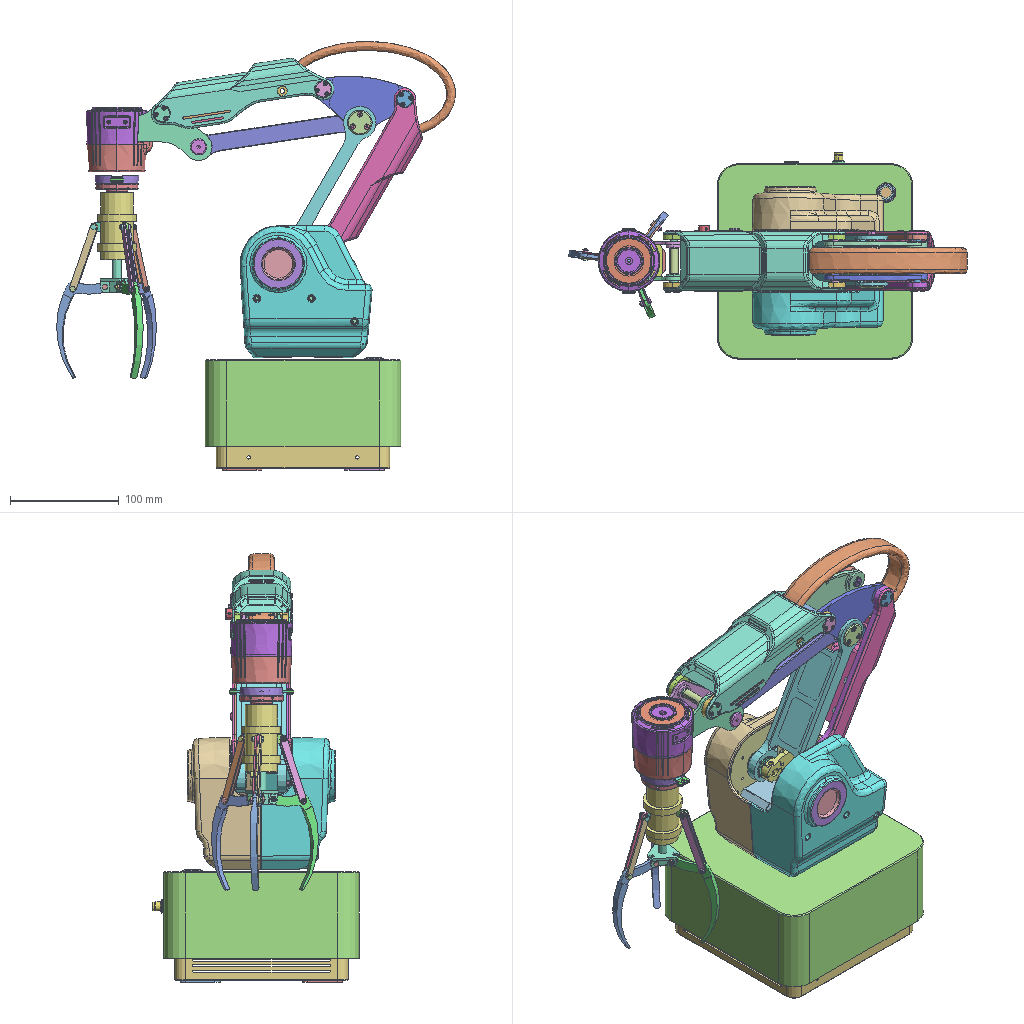Assembly | NX | 116 different items | 163 placed | box 367 x 190 x 394 mm
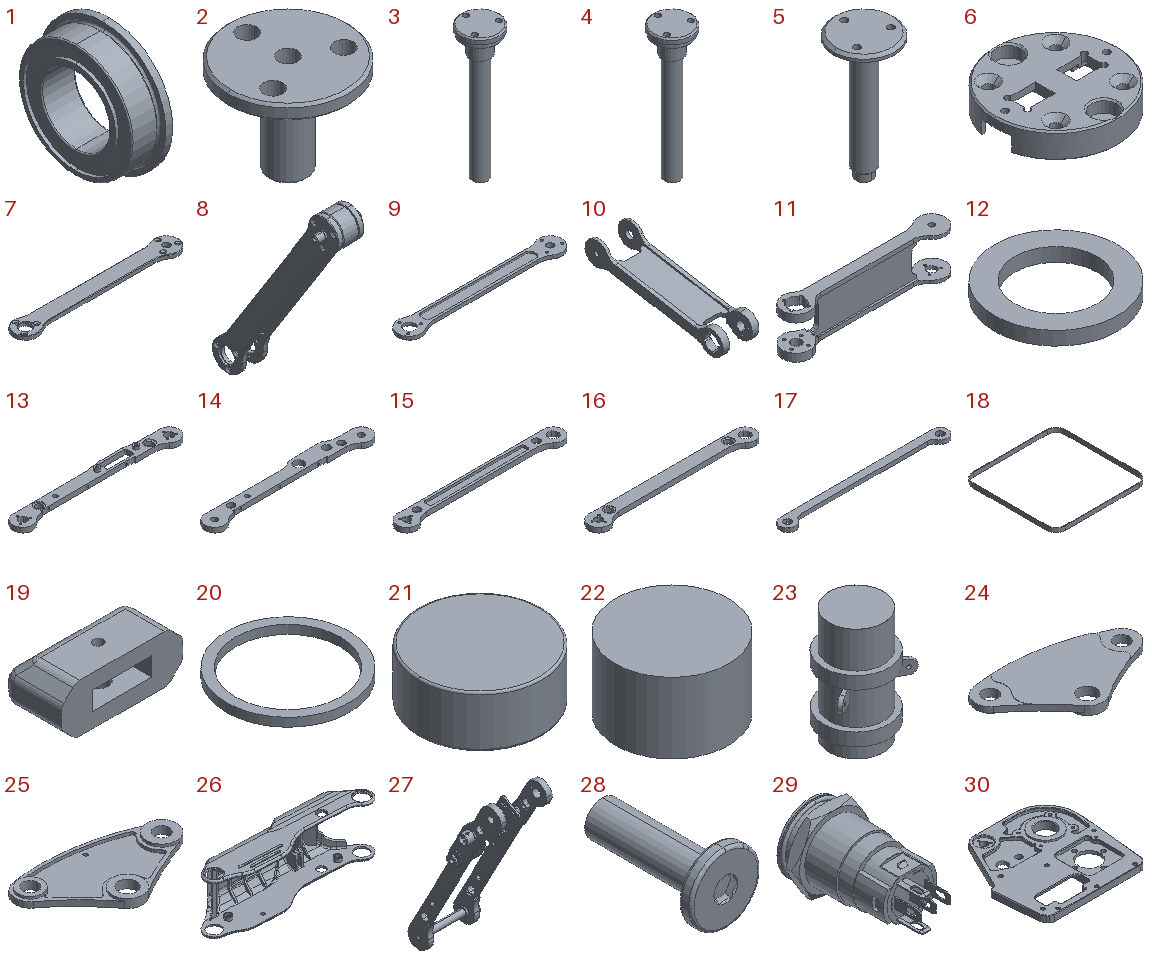Parts list (item | name | quantity | parent item | size | volume | features):
1 | - | x1 | - | 3 x 11.2 x 11.2 mm | 145.175 mm3 | features BREP 1
2 | - | x1 | in 68 | 12.5 x 12.5 x 10.2 mm | 244.426 mm3 | features BREP 1
3 | - | x1 | in 68 | 15 x 15 x 52.6 mm | 2030 mm3 | features BREP 1
4 | - | x1 | in 27 | 15 x 15 x 52.6 mm | 2030 mm3 | features BREP 1
5 | - | x1 | in 68 | 23 x 23 x 48 mm | 3023 mm3 | features BREP 1
6 | - | x1 | in 65 | 40 x 40 x 8 mm | 4406 mm3 | features BREP 1
7 | - | x1 | in 8 | 175 x 25 x 4 mm | 8666 mm3 | features REPLACE_FACE 3, BREP 1
8 | - | x1 | in 68 | 36.8 x 104.994 x 151.889 mm | 23605 mm3 | features BREP 3, REPLACE_FACE 3
9 | - | x1 | in 8 | 175 x 25 x 4 mm | 8666 mm3 | features BREP 1
10 | - | x1 | in 68 | 49 x 177.857 x 55.267 mm | 37344 mm3 | features BREP 2
11 | - | x1 | in 10 | 180 x 30 x 46 mm | 37069 mm3 | features BREP 1
12 | - | x1 | - | 9 x 9 x 1 mm | 35.343 mm3 | features BREP 1
13 | - | x1 | in 27 | 170 x 22.394 x 8 mm | 9194 mm3 | features BREP 1
14 | - | x1 | in 27 | 170 x 24.378 x 5 mm | 10473 mm3 | features BREP 1
15 | - | x1 | in 68 | 169.999 x 20 x 5 mm | 8700 mm3 | features BREP 1
16 | - | x1 | in 68 | 170 x 20 x 5 mm | 8700 mm3 | features BREP 1
17 | - | x1 | in 68 | 165 x 15 x 4 mm | 5289 mm3 | features BREP 1
18 | - | x1 | in 49 | 176 x 176 x 7.9 mm | 5293 mm3 | features BREP 1
19 | - | x2 | in 65 | 12.444 x 5.907 x 4.95 mm | 254.253 mm3 | features BREP 1
20 | - | x1 | - | 23.91 x 23.91 x 1.67 mm | 211.991 mm3 | features BREP 1
21 | - | x1 | - | 6 x 6 x 2.5 mm | 70.606 mm3 | features BREP 1
22 | - | x1 | - | 8 x 8 x 5 mm | 251.327 mm3 | features BREP 1
23 | - | x1 | in 74 | 43.868 x 42.75 x 62.001 mm | 27511 mm3 | features EXTRUDE 9, DATUM_CSYS 8, SKETCH 7, EXTRACT_STRING 6, HOLE PACKAGE 3, SIMPLE HOLE 3, Instance Feature 2, BREP 1, DATUM_PLANE 1, LINKED_FACE 1, Pattern Feature 1, SHELL 1, UNITE 1
24 | - | x1 | in 68 | 94.779 x 53.231 x 5.8 mm | 8618 mm3 | features BREP 1
25 | - | x1 | in 68 | 94.779 x 53.231 x 5.8 mm | 8608 mm3 | features BREP 1
26 | - | x1 | in 68 | 169.834 x 48.221 x 55.5 mm | 47491 mm3 | features BREP 5, DATUM_CSYS 4, SKETCH 4, DELETE FACE 3, EXTRUDE 2
27 | - | x1 | in 68 | 60.8 x 89.643 x 152.852 mm | 26403 mm3 | features BREP 185
28 | - | x4 | in 67 | 5 x 8.9 x 5 mm | 55.675 mm3 | features BREP 1
29 | - | x1 | in 49 | 21.708 x 35 x 18.8 mm | 5416 mm3 | features BREP 6
30 | - | x1 | in 68 | 113.03 x 111.071 x 8.2 mm | 44822 mm3 | features BREP 1
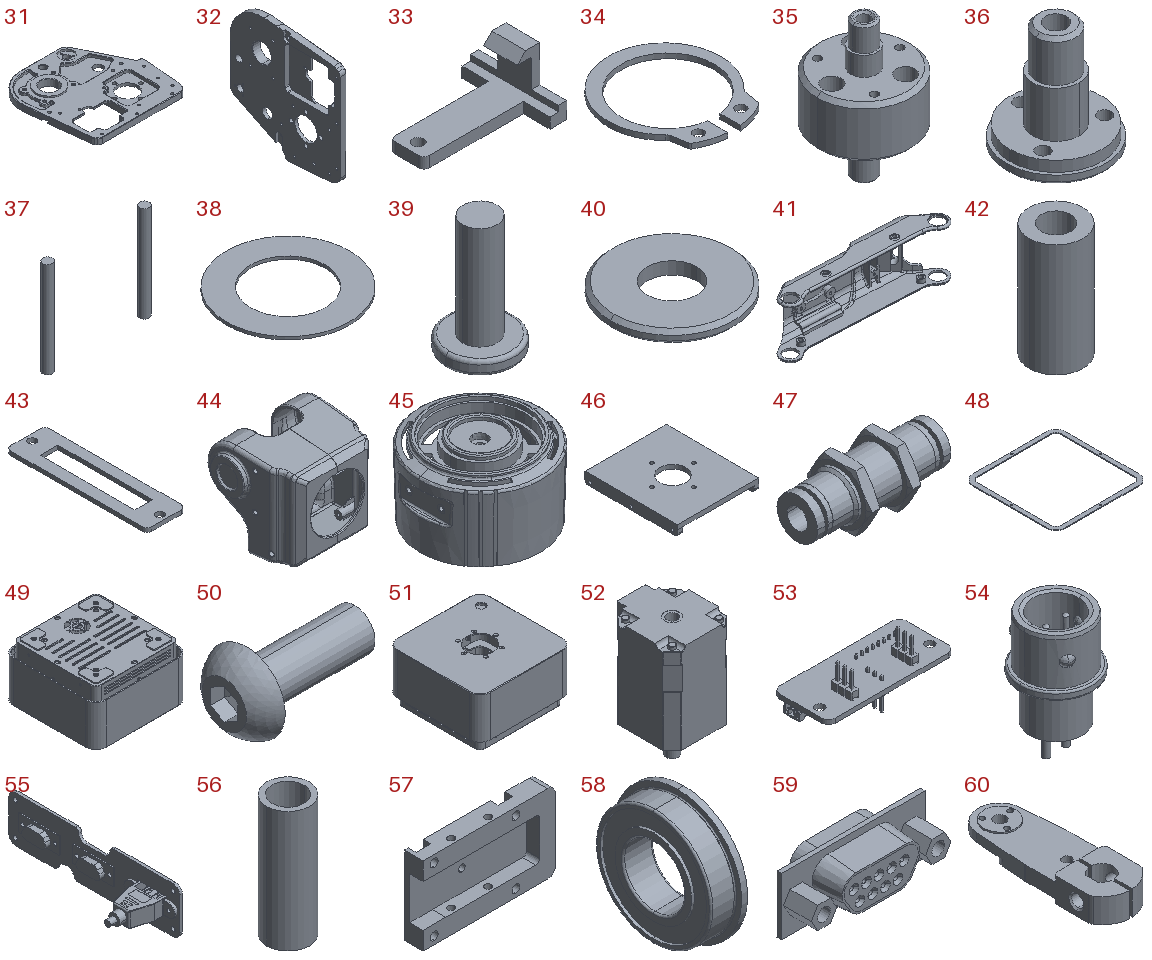31 | - | x1 | in 32 | 113.061 x 111.064 x 8.2 mm | 45327 mm3 | features BREP 1
32 | - | x1 | in 68 | 8.2 x 111.064 x 113.061 mm | 45327 mm3 | features BREP 1
33 | - | x2 | in 65 | 20.555 x 15.6 x 9.4 mm | 383.369 mm3 | features BREP 2, REPLACE_FACE 1, UNITE 1
34 | - | x1 | in 65 | 22.5 x 25.161 x 1 mm | 153.893 mm3 | features BREP 1
35 | - | x1 | in 8 | 25 x 25 x 36.8 mm | 6273 mm3 | features BREP 1
36 | - | x4 | in 68 | 15 x 15 x 16.2 mm | 821.71 mm3 | features BREP 1
37 | - | x1 | in 65 | 22.254 x 2 x 20 mm | 125.664 mm3 | features BREP 2
38 | - | x1 | in 65 | 42.2 x 42.2 x 1 mm | 887.963 mm3 | features BREP 1
39 | - | x15 | in 67 | 4 x 4 x 6.8 mm | 27.69 mm3 | features BREP 1
40 | - | x1 | - | 10 x 10 x 1 mm | 63.203 mm3 | features BREP 1
41 | - | x1 | in 68 | 169.834 x 45.304 x 55 mm | 40622 mm3 | features BREP 3
42 | - | x1 | in 68 | 11 x 11 x 23 mm | 1525 mm3 | features BREP 1
43 | - | x1 | in 67 | 16 x 58 x 1.6 mm | 998.284 mm3 | features BREP 1
44 | - | x1 | in 68 | 136.184 x 121.469 x 121.428 mm | 181259 mm3 | features BREP 6
45 | - | x1 | in 65 | 56.842 x 56.842 x 34.1 mm | 13969 mm3 | features BREP 5
46 | - | x1 | in 68 | 77.6 x 88.919 x 10.2 mm | 30243 mm3 | features BREP 1
47 | - | x1 | in 49 | 26 x 12.702 x 11 mm | 1290 mm3 | features BREP 3
48 | - | x1 | in 67 | 176.2 x 176.2 x 1.5 mm | 7641 mm3 | features BREP 1
49 | - | x1 | in 67 | - | 318860 mm3 | features BREP 63
50 | - | x1 | in 66 | 9.65 x 5.7 x 5.7 mm | 82.821 mm3 | features BREP 1
51 | - | x1 | in 49 | 180 x 180.4 x 102 mm | 289321 mm3 | features BREP 44
52 | - | x2 | in 68 | 42 x 48 x 79 mm | 100479 mm3 | features BREP 1
53 | - | x1 | in 27 | 45.595 x 20 x 18.599 mm | 1843 mm3 | features BREP 177
54 | - | x1 | in 27 | 11.1 x 11.1 x 18.7 mm | 715.454 mm3 | features BREP 4
55 | - | x1 | in 49 | 39.87 x 130 x 35 mm | 15905 mm3 | features BREP 8
56 | - | x1 | in 67 | 8.1 x 8.1 x 23 mm | 513.022 mm3 | features BREP 1
57 | - | x1 | in 66 | 50.135 x 8.5 x 29.6 mm | 6295 mm3 | features BREP 1
58 | - | x6 | in 68 | 5 x 21 x 21 mm | 978.232 mm3 | features BREP 1
59 | - | x2 | in 55 | 31.31 x 11.07 x 12.55 mm | 1882 mm3 | features BREP 1
60 | - | x1 | in 68 | 17.477 x 52.487 x 8.4 mm | 3967 mm3 | features BREP 1
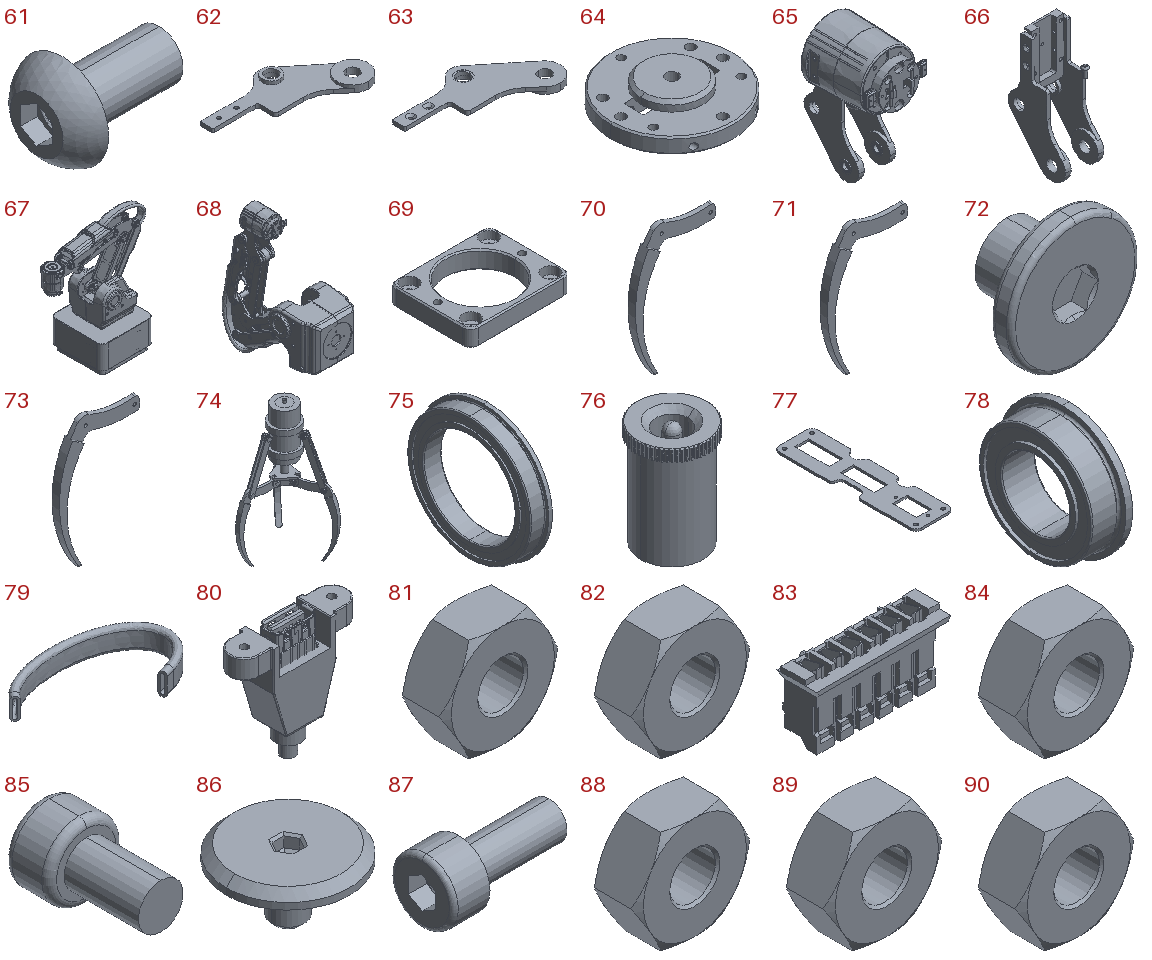61 | - | x4 | in 10 | 7.65 x 5.7 x 5.7 mm | 68.684 mm3 | features BREP 1
62 | - | x1 | in 66 | 104.242 x 53.12 x 5.7 mm | 7739 mm3 | features BREP 2, Delete Body 1, REPLACE_FACE 1
63 | - | x1 | in 66 | 104.242 x 53.12 x 5.7 mm | 7724 mm3 | features BREP 2, Delete Body 1
64 | - | x1 | in 67 | 40 x 40 x 8 mm | 5675 mm3 | features BREP 1
65 | - | x1 | in 68 | 59.043 x 79.079 x 115.958 mm | 60024 mm3 | features BREP 23, Delete Body 2, REPLACE_FACE 2, UNITE 1
66 | - | x1 | in 65 | 35.6 x 56.422 x 107.242 mm | 21841 mm3 | features BREP 6, Delete Body 2, REPLACE_FACE 1
67 | - | x1 | - | - | 1159174 mm3 | features BREP 318, REPLACE_FACE 5, DATUM_CSYS 4, SKETCH 4, DELETE FACE 3, Delete Body 2, EXTRUDE 2, UNITE 1
68 | - | x1 | in 67 | - | 823065 mm3 | features BREP 245, REPLACE_FACE 5, DATUM_CSYS 4, SKETCH 4, DELETE FACE 3, Delete Body 2, EXTRUDE 2, UNITE 1
69 | - | x1 | in 65 | 39.409 x 32 x 6.9 mm | 4078 mm3 | features BREP 1
70 | - | x1 | in 74 | 50.786 x 11.051 x 88.315 mm | 3379 mm3 | features DATUM_CSYS 4, EXTRUDE 3, SKETCH 3, CPROJ 2, BLEND 1
71 | - | x1 | in 74 | 50.786 x 11.051 x 88.315 mm | 3379 mm3 | features DATUM_CSYS 4, EXTRUDE 3, SKETCH 3, CPROJ 2, BLEND 1
72 | - | x4 | in 67 | 8.1 x 4.3 x 8.1 mm | 98.194 mm3 | features BREP 1
73 | - | x1 | in 74 | 50.786 x 11.051 x 88.315 mm | 3379 mm3 | features DATUM_CSYS 4, EXTRUDE 3, SKETCH 3, CPROJ 2, BLEND 1
74 | - | x1 | - | 91.731 x 98.46 x 173.883 mm | 50064 mm3 | features BREP 26, DATUM_CSYS 26, EXTRUDE 23, SKETCH 21, CPROJ 8, EXTRACT_STRING 6, BLEND 4, HOLE PACKAGE 3, SIMPLE HOLE 3, UNITE 3, DATUM_PLANE 2, EXTRACT_BODY 2, Instance Feature 2, Delete Body 1, LINKED_FACE 1, Pattern Feature 1, Pattern Geometry 1, SHELL 1
75 | - | x2 | in 65 | 4 x 28.5 x 28.5 mm | 1002 mm3 | features BREP 1
76 | - | x1 | in 49 | 12.424 x 12.424 x 18.4 mm | 1636 mm3 | features BREP 1
77 | - | x1 | in 55 | 35 x 130 x 2 mm | 6211 mm3 | features BREP 1
78 | - | x4 | in 65 | 3 x 11.2 x 11.2 mm | 145.175 mm3 | features BREP 1
79 | - | x1 | in 68 | 150.882 x 88.437 x 24 mm | 23411 mm3 | features BREP 1
80 | - | x1 | in 55 | 39 x 11.5 x 39.2 mm | 5931 mm3 | features BREP 6
81 | - | x1 | in 74 | 5.196 x 2 x 4.5 mm | 28.526 mm3 | features BREP 1
82 | - | x1 | in 74 | 5.196 x 2 x 4.5 mm | 28.526 mm3 | features BREP 1
83 | - | x1 | - | 13.8 x 4.5 x 6.85 mm | 132.945 mm3 | features BREP 7
84 | - | x1 | in 74 | 5.196 x 2 x 4.5 mm | 28.526 mm3 | features BREP 1
85 | - | x6 | in 67 | 5 x 8 x 5 mm | 87.225 mm3 | features BREP 1
86 | - | x4 | in 68 | 15 x 15 x 8 mm | 442.432 mm3 | features BREP 1
87 | - | x1 | in 67 | 14 x 7 x 7 mm | 260.941 mm3 | features BREP 1
88 | - | x1 | in 74 | 5.196 x 2 x 4.5 mm | 28.526 mm3 | features BREP 1
89 | - | x1 | in 74 | 5.196 x 2 x 4.5 mm | 28.526 mm3 | features BREP 1
90 | - | x1 | in 74 | 5.196 x 2 x 4.5 mm | 28.526 mm3 | features BREP 1
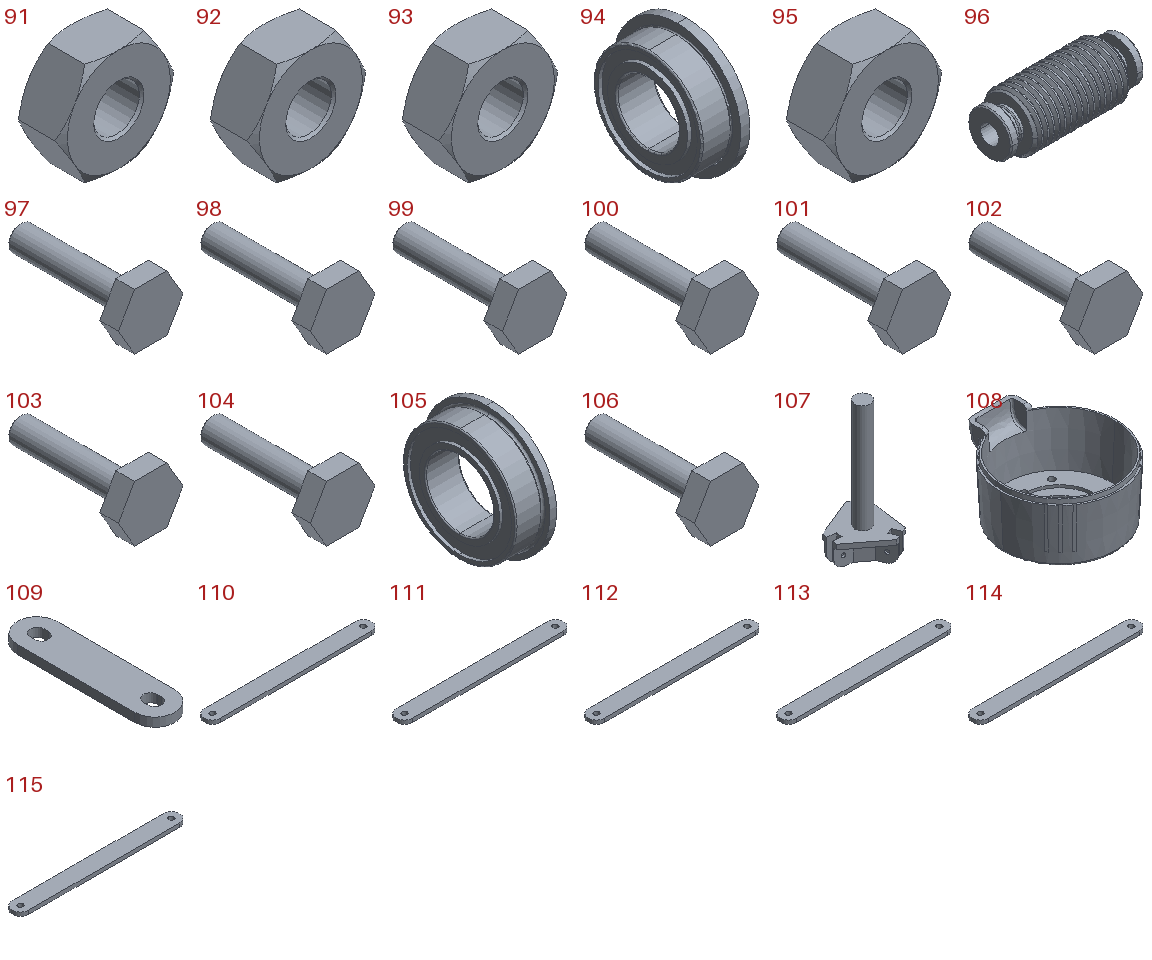91 | - | x1 | in 74 | 5.196 x 2 x 4.5 mm | 28.526 mm3 | features BREP 1
92 | - | x1 | in 74 | 5.196 x 2 x 4.5 mm | 28.526 mm3 | features BREP 1
93 | - | x1 | in 74 | 5.196 x 2 x 4.5 mm | 28.526 mm3 | features BREP 1
94 | - | x1 | - | 2.5 x 8.2 x 8.2 mm | 67.176 mm3 | features BREP 1
95 | - | x1 | - | 5.196 x 2 x 4.5 mm | 28.526 mm3 | features BREP 1
96 | - | x1 | in 27 | 29 x 12 x 12 mm | 2150 mm3 | features BREP 1
97 | - | x1 | in 74 | 5.196 x 10.5 x 4.5 mm | 54.581 mm3 | features BREP 1
98 | - | x1 | in 74 | 5.196 x 10.5 x 4.5 mm | 54.581 mm3 | features BREP 1
99 | - | x1 | in 74 | 5.196 x 10.5 x 4.5 mm | 54.581 mm3 | features BREP 1
100 | - | x1 | in 74 | 5.196 x 10.5 x 4.5 mm | 54.581 mm3 | features BREP 1
101 | - | x1 | in 74 | 5.196 x 10.5 x 4.5 mm | 54.581 mm3 | features BREP 1
102 | - | x1 | in 74 | 5.196 x 10.5 x 4.5 mm | 54.581 mm3 | features BREP 1
103 | - | x1 | in 74 | 5.196 x 10.5 x 4.5 mm | 54.581 mm3 | features BREP 1
104 | - | x1 | in 74 | 5.196 x 10.5 x 4.5 mm | 54.581 mm3 | features BREP 1
105 | - | x1 | - | 3 x 11.2 x 11.2 mm | 145.175 mm3 | features BREP 1
106 | - | x1 | in 74 | 5.196 x 10.5 x 4.5 mm | 54.581 mm3 | features BREP 1
107 | - | x1 | in 74 | 27.712 x 29.745 x 67.5 mm | 4749 mm3 | features DATUM_CSYS 6, EXTRUDE 5, SKETCH 5, CPROJ 2, EXTRACT_BODY 2, UNITE 2, BLEND 1, BREP 1, DATUM_PLANE 1, Delete Body 1, Pattern Geometry 1
108 | - | x1 | in 65 | 55.272 x 60.87 x 29.488 mm | 10698 mm3 | features BREP 1
109 | - | x1 | in 67 | 9.123 x 36.123 x 2 mm | 578.449 mm3 | features BREP 1
110 | - | x1 | in 74 | 66.5 x 6.5 x 1.5 mm | 625.35 mm3 | features BREP 1
111 | - | x1 | in 74 | 66.5 x 6.5 x 1.5 mm | 625.35 mm3 | features BREP 1
112 | - | x1 | in 74 | 66.5 x 6.5 x 1.5 mm | 625.35 mm3 | features BREP 1
113 | - | x1 | in 74 | 66.5 x 6.5 x 1.5 mm | 625.35 mm3 | features BREP 1
114 | - | x1 | in 74 | 66.5 x 6.5 x 1.5 mm | 625.35 mm3 | features BREP 1
115 | - | x1 | in 74 | 66.5 x 6.5 x 1.5 mm | 625.35 mm3 | features BREP 1
116 | 连接座 | x1 | - | - | - | -
Mates (type | each side: item.copy, entity, surface, feature):
Touch | 110.1 | 70.1
Touch | 97.1 | 111.1
Touch | 98.1 | 111.1
Touch | 99.1 | 107.1
Touch | 81.1 | 97.1
Distance | 111.1 | 23.1
Distance | 81.1 | 23.1
Touch | 82.1 | 98.1
Touch | 82.1 | 110.1
Touch | 84.1 | 99.1
Touch | 84.1 | 107.1
Touch | 100.1 | 113.1 | 2 times
Touch | 101.1 | 113.1 | 2 times
Touch | 102.1 | 107.1 | 2 times
Touch | 88.1 | 100.1
Touch | 88.1 | 112.1
Touch | 89.1 | 101.1
Touch | 89.1 | 112.1
Touch | 90.1 | 102.1
Touch | 90.1 | 107.1
Touch | 73.1 | 107.1
Distance | 73.1 | 107.1
Touch | 114.1 | 23.1
Touch | 114.1 | 73.1
Distance | 114.1 | 73.1
Touch | 115.1 | 23.1
Touch | 115.1 | 73.1 | 2 times
Touch | 103.1 | 23.1
Touch | 103.1 | 115.1
Touch | 104.1 | 115.1 | 2 times
Touch | 106.1 | 107.1 | 2 times
Touch | 91.1 | 103.1
Touch | 91.1 | 114.1
Touch | 92.1 | 104.1
Touch | 92.1 | 114.1
Touch | 93.1 | 106.1
Touch | 93.1 | 107.1